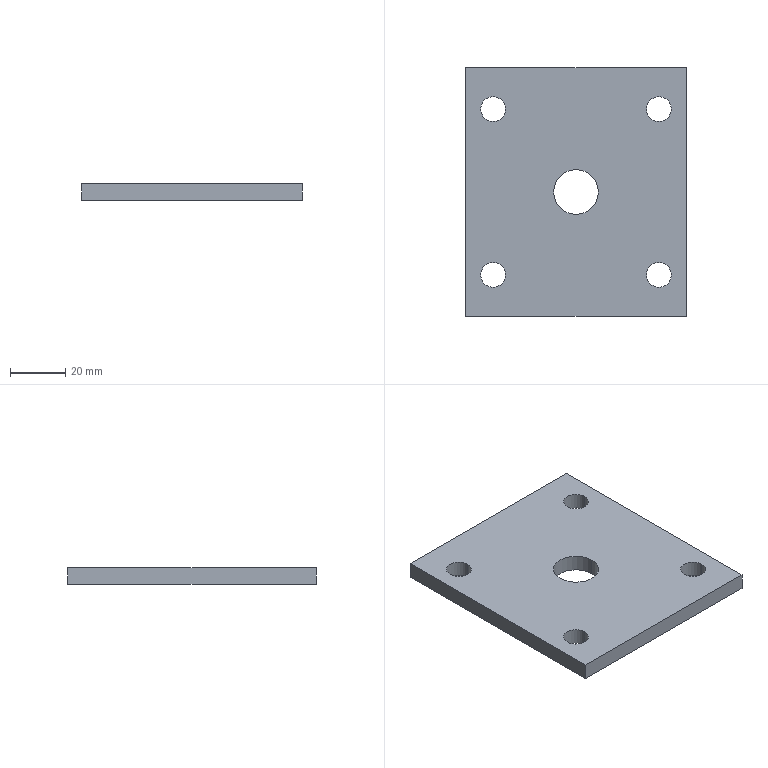Part | SolidWorks | features Extrusion 1, ICE 1 | 1 solid | 16 faces | box 80 x 90 x 6 mm | volume 40436 mm3 | cylinder 10 | plane 6 | commonest cylinder face diameters 9 x8 16.2 x2
STEP:
#1=CARTESIAN_POINT('',(-34.5,30.,-3.));
#2=VERTEX_POINT('',#1);
#3=CARTESIAN_POINT('',(-25.5,30.,-3.));
#4=VERTEX_POINT('',#3);
#5=CARTESIAN_POINT('',(-30.,30.,-3.));
#6=DIRECTION('',(0.,0.,1.));
#7=DIRECTION('',(1.,0.,0.));
#8=AXIS2_PLACEMENT_3D('',#5,#6,#7);
#9=CIRCLE('',#8,4.5);
#10=EDGE_CURVE('',#2,#4,#9,.T.);
#11=ORIENTED_EDGE('',*,*,#10,.F.);
#12=CARTESIAN_POINT('',(-34.5,30.,3.));
#13=VERTEX_POINT('',#12);
#14=CARTESIAN_POINT('',(-34.5,30.,-13.));
#15=DIRECTION('',(0.,0.,1.));
#16=VECTOR('',#15,1000.);
#17=LINE('',#14,#16);
#18=EDGE_CURVE('',#2,#13,#17,.T.);
#19=ORIENTED_EDGE('',*,*,#18,.T.);
#20=CARTESIAN_POINT('',(-25.5,30.,3.));
#21=VERTEX_POINT('',#20);
#22=CARTESIAN_POINT('',(-30.,30.,3.));
#23=DIRECTION('',(0.,0.,1.));
#24=DIRECTION('',(1.,0.,0.));
#25=AXIS2_PLACEMENT_3D('',#22,#23,#24);
#26=CIRCLE('',#25,4.5);
#27=EDGE_CURVE('',#13,#21,#26,.T.);
#28=ORIENTED_EDGE('',*,*,#27,.T.);
#29=CARTESIAN_POINT('',(-25.5,30.,-13.));
#30=DIRECTION('',(0.,0.,1.));
#31=VECTOR('',#30,1000.);
#32=LINE('',#29,#31);
#33=EDGE_CURVE('',#4,#21,#32,.T.);
#34=ORIENTED_EDGE('',*,*,#33,.F.);
#35=EDGE_LOOP('',(#11,#19,#28,#34));
#36=FACE_OUTER_BOUND('',#35,.T.);
#37=CARTESIAN_POINT('',(-30.,30.,-13.));
#38=DIRECTION('',(0.,0.,1.));
#39=DIRECTION('',(1.,0.,0.));
#40=AXIS2_PLACEMENT_3D('',#37,#38,#39);
#41=CYLINDRICAL_SURFACE('',#40,4.5);
#42=ADVANCED_FACE('',(#36),#41,.F.);
#43=CARTESIAN_POINT('',(25.5,-30.,-3.));
#44=VERTEX_POINT('',#43);
#45=CARTESIAN_POINT('',(34.5,-30.,-3.));
#46=VERTEX_POINT('',#45);
#47=CARTESIAN_POINT('',(30.,-30.,-3.));
#48=DIRECTION('',(0.,0.,1.));
#49=DIRECTION('',(1.,0.,0.));
#50=AXIS2_PLACEMENT_3D('',#47,#48,#49);
#51=CIRCLE('',#50,4.5);
#52=EDGE_CURVE('',#44,#46,#51,.T.);
#53=ORIENTED_EDGE('',*,*,#52,.F.);
#54=CARTESIAN_POINT('',(25.5,-30.,3.));
#55=VERTEX_POINT('',#54);
#56=CARTESIAN_POINT('',(25.5,-30.,-13.));
#57=DIRECTION('',(0.,0.,1.));
#58=VECTOR('',#57,1000.);
#59=LINE('',#56,#58);
#60=EDGE_CURVE('',#44,#55,#59,.T.);
#61=ORIENTED_EDGE('',*,*,#60,.T.);
#62=CARTESIAN_POINT('',(34.5,-30.,3.));
#63=VERTEX_POINT('',#62);
#64=CARTESIAN_POINT('',(30.,-30.,3.));
#65=DIRECTION('',(0.,0.,1.));
#66=DIRECTION('',(1.,0.,0.));
#67=AXIS2_PLACEMENT_3D('',#64,#65,#66);
#68=CIRCLE('',#67,4.5);
#69=EDGE_CURVE('',#55,#63,#68,.T.);
#70=ORIENTED_EDGE('',*,*,#69,.T.);
#71=CARTESIAN_POINT('',(34.5,-30.,-13.));
#72=DIRECTION('',(0.,0.,1.));
#73=VECTOR('',#72,1000.);
#74=LINE('',#71,#73);
#75=EDGE_CURVE('',#46,#63,#74,.T.);
#76=ORIENTED_EDGE('',*,*,#75,.F.);
#77=EDGE_LOOP('',(#53,#61,#70,#76));
#78=FACE_OUTER_BOUND('',#77,.T.);
#79=CARTESIAN_POINT('',(30.,-30.,-13.));
#80=DIRECTION('',(0.,0.,1.));
#81=DIRECTION('',(1.,0.,0.));
#82=AXIS2_PLACEMENT_3D('',#79,#80,#81);
#83=CYLINDRICAL_SURFACE('',#82,4.5);
#84=ADVANCED_FACE('',(#78),#83,.F.);
#85=CARTESIAN_POINT('',(25.5,30.,-3.));
#86=VERTEX_POINT('',#85);
#87=CARTESIAN_POINT('',(34.5,30.,-3.));
#88=VERTEX_POINT('',#87);
#89=CARTESIAN_POINT('',(30.,30.,-3.));
#90=DIRECTION('',(0.,0.,1.));
#91=DIRECTION('',(1.,0.,0.));
#92=AXIS2_PLACEMENT_3D('',#89,#90,#91);
#93=CIRCLE('',#92,4.5);
#94=EDGE_CURVE('',#86,#88,#93,.T.);
#95=ORIENTED_EDGE('',*,*,#94,.F.);
#96=CARTESIAN_POINT('',(25.5,30.,3.));
#97=VERTEX_POINT('',#96);
#98=CARTESIAN_POINT('',(25.5,30.,-13.));
#99=DIRECTION('',(0.,0.,1.));
#100=VECTOR('',#99,1000.);
#101=LINE('',#98,#100);
#102=EDGE_CURVE('',#86,#97,#101,.T.);
#103=ORIENTED_EDGE('',*,*,#102,.T.);
#104=CARTESIAN_POINT('',(34.5,30.,3.));
#105=VERTEX_POINT('',#104);
#106=CARTESIAN_POINT('',(30.,30.,3.));
#107=DIRECTION('',(0.,0.,1.));
#108=DIRECTION('',(1.,0.,0.));
#109=AXIS2_PLACEMENT_3D('',#106,#107,#108);
#110=CIRCLE('',#109,4.5);
#111=EDGE_CURVE('',#97,#105,#110,.T.);
#112=ORIENTED_EDGE('',*,*,#111,.T.);
#113=CARTESIAN_POINT('',(34.5,30.,-13.));
#114=DIRECTION('',(0.,0.,1.));
#115=VECTOR('',#114,1000.);
#116=LINE('',#113,#115);
#117=EDGE_CURVE('',#88,#105,#116,.T.);
#118=ORIENTED_EDGE('',*,*,#117,.F.);
#119=EDGE_LOOP('',(#95,#103,#112,#118));
#120=FACE_OUTER_BOUND('',#119,.T.);
#121=CARTESIAN_POINT('',(30.,30.,-13.));
#122=DIRECTION('',(0.,0.,1.));
#123=DIRECTION('',(1.,0.,0.));
#124=AXIS2_PLACEMENT_3D('',#121,#122,#123);
#125=CYLINDRICAL_SURFACE('',#124,4.5);
#126=ADVANCED_FACE('',(#120),#125,.F.);
#127=CARTESIAN_POINT('',(-8.1,0.,-3.));
#128=VERTEX_POINT('',#127);
#129=CARTESIAN_POINT('',(8.1,0.,-3.));
#130=VERTEX_POINT('',#129);
#131=CARTESIAN_POINT('',(0.,0.,-3.));
#132=DIRECTION('',(0.,0.,1.));
#133=DIRECTION('',(1.,0.,0.));
#134=AXIS2_PLACEMENT_3D('',#131,#132,#133);
#135=CIRCLE('',#134,8.1);
#136=EDGE_CURVE('',#128,#130,#135,.T.);
#137=ORIENTED_EDGE('',*,*,#136,.F.);
#138=CARTESIAN_POINT('',(-8.1,0.,3.));
#139=VERTEX_POINT('',#138);
#140=CARTESIAN_POINT('',(-8.1,0.,-13.));
#141=DIRECTION('',(0.,0.,1.));
#142=VECTOR('',#141,1000.);
#143=LINE('',#140,#142);
#144=EDGE_CURVE('',#128,#139,#143,.T.);
#145=ORIENTED_EDGE('',*,*,#144,.T.);
#146=CARTESIAN_POINT('',(8.1,0.,3.));
#147=VERTEX_POINT('',#146);
#148=CARTESIAN_POINT('',(0.,0.,3.));
#149=DIRECTION('',(0.,0.,1.));
#150=DIRECTION('',(1.,0.,0.));
#151=AXIS2_PLACEMENT_3D('',#148,#149,#150);
#152=CIRCLE('',#151,8.1);
#153=EDGE_CURVE('',#139,#147,#152,.T.);
#154=ORIENTED_EDGE('',*,*,#153,.T.);
#155=CARTESIAN_POINT('',(8.1,0.,-13.));
#156=DIRECTION('',(0.,0.,1.));
#157=VECTOR('',#156,1000.);
#158=LINE('',#155,#157);
#159=EDGE_CURVE('',#130,#147,#158,.T.);
#160=ORIENTED_EDGE('',*,*,#159,.F.);
#161=EDGE_LOOP('',(#137,#145,#154,#160));
#162=FACE_OUTER_BOUND('',#161,.T.);
#163=CARTESIAN_POINT('',(0.,0.,-13.));
#164=DIRECTION('',(0.,0.,1.));
#165=DIRECTION('',(1.,0.,0.));
#166=AXIS2_PLACEMENT_3D('',#163,#164,#165);
#167=CYLINDRICAL_SURFACE('',#166,8.1);
#168=ADVANCED_FACE('',(#162),#167,.F.);
#169=CARTESIAN_POINT('',(-34.5,-30.,-3.));
#170=VERTEX_POINT('',#169);
#171=CARTESIAN_POINT('',(-25.5,-30.,-3.));
#172=VERTEX_POINT('',#171);
#173=CARTESIAN_POINT('',(-30.,-30.,-3.));
#174=DIRECTION('',(0.,0.,1.));
#175=DIRECTION('',(1.,0.,0.));
#176=AXIS2_PLACEMENT_3D('',#173,#174,#175);
#177=CIRCLE('',#176,4.5);
#178=EDGE_CURVE('',#170,#172,#177,.T.);
#179=ORIENTED_EDGE('',*,*,#178,.F.);
#180=CARTESIAN_POINT('',(-34.5,-30.,3.));
#181=VERTEX_POINT('',#180);
#182=CARTESIAN_POINT('',(-34.5,-30.,-13.));
#183=DIRECTION('',(0.,0.,1.));
#184=VECTOR('',#183,1000.);
#185=LINE('',#182,#184);
#186=EDGE_CURVE('',#170,#181,#185,.T.);
#187=ORIENTED_EDGE('',*,*,#186,.T.);
#188=CARTESIAN_POINT('',(-25.5,-30.,3.));
#189=VERTEX_POINT('',#188);
#190=CARTESIAN_POINT('',(-30.,-30.,3.));
#191=DIRECTION('',(0.,0.,1.));
#192=DIRECTION('',(1.,0.,0.));
#193=AXIS2_PLACEMENT_3D('',#190,#191,#192);
#194=CIRCLE('',#193,4.5);
#195=EDGE_CURVE('',#181,#189,#194,.T.);
#196=ORIENTED_EDGE('',*,*,#195,.T.);
#197=CARTESIAN_POINT('',(-25.5,-30.,-13.));
#198=DIRECTION('',(0.,0.,1.));
#199=VECTOR('',#198,1000.);
#200=LINE('',#197,#199);
#201=EDGE_CURVE('',#172,#189,#200,.T.);
#202=ORIENTED_EDGE('',*,*,#201,.F.);
#203=EDGE_LOOP('',(#179,#187,#196,#202));
#204=FACE_OUTER_BOUND('',#203,.T.);
#205=CARTESIAN_POINT('',(-30.,-30.,-13.));
#206=DIRECTION('',(0.,0.,1.));
#207=DIRECTION('',(1.,0.,0.));
#208=AXIS2_PLACEMENT_3D('',#205,#206,#207);
#209=CYLINDRICAL_SURFACE('',#208,4.5);
#210=ADVANCED_FACE('',(#204),#209,.F.);
#211=CARTESIAN_POINT('',(-40.,45.,3.));
#212=VERTEX_POINT('',#211);
#213=CARTESIAN_POINT('',(-40.,-45.,3.));
#214=VERTEX_POINT('',#213);
#215=CARTESIAN_POINT('',(-40.,45.,3.));
#216=DIRECTION('',(0.,-1.,0.));
#217=VECTOR('',#216,1000.);
#218=LINE('',#215,#217);
#219=EDGE_CURVE('',#212,#214,#218,.T.);
#220=ORIENTED_EDGE('',*,*,#219,.F.);
#221=CARTESIAN_POINT('',(-40.,45.,-3.));
#222=VERTEX_POINT('',#221);
#223=CARTESIAN_POINT('',(-40.,45.,-3.));
#224=DIRECTION('',(0.,0.,1.));
#225=VECTOR('',#224,1000.);
#226=LINE('',#223,#225);
#227=EDGE_CURVE('',#222,#212,#226,.T.);
#228=ORIENTED_EDGE('',*,*,#227,.F.);
#229=CARTESIAN_POINT('',(-40.,-45.,-3.));
#230=VERTEX_POINT('',#229);
#231=CARTESIAN_POINT('',(-40.,45.,-3.));
#232=DIRECTION('',(0.,-1.,0.));
#233=VECTOR('',#232,1000.);
#234=LINE('',#231,#233);
#235=EDGE_CURVE('',#222,#230,#234,.T.);
#236=ORIENTED_EDGE('',*,*,#235,.T.);
#237=CARTESIAN_POINT('',(-40.,-45.,-3.));
#238=DIRECTION('',(0.,0.,1.));
#239=VECTOR('',#238,1000.);
#240=LINE('',#237,#239);
#241=EDGE_CURVE('',#230,#214,#240,.T.);
#242=ORIENTED_EDGE('',*,*,#241,.T.);
#243=EDGE_LOOP('',(#220,#228,#236,#242));
#244=FACE_OUTER_BOUND('',#243,.T.);
#245=CARTESIAN_POINT('',(-40.,45.,-3.));
#246=DIRECTION('',(-1.,0.,0.));
#247=DIRECTION('',(0.,0.,1.));
#248=AXIS2_PLACEMENT_3D('',#245,#246,#247);
#249=PLANE('',#248);
#250=ADVANCED_FACE('',(#244),#249,.T.);
#251=CARTESIAN_POINT('',(40.,45.,3.));
#252=VERTEX_POINT('',#251);
#253=CARTESIAN_POINT('',(40.,45.,3.));
#254=DIRECTION('',(-1.,0.,0.));
#255=VECTOR('',#254,1000.);
#256=LINE('',#253,#255);
#257=EDGE_CURVE('',#252,#212,#256,.T.);
#258=ORIENTED_EDGE('',*,*,#257,.F.);
#259=CARTESIAN_POINT('',(40.,45.,-3.));
#260=VERTEX_POINT('',#259);
#261=CARTESIAN_POINT('',(40.,45.,-3.));
#262=DIRECTION('',(0.,0.,1.));
#263=VECTOR('',#262,1000.);
#264=LINE('',#261,#263);
#265=EDGE_CURVE('',#260,#252,#264,.T.);
#266=ORIENTED_EDGE('',*,*,#265,.F.);
#267=CARTESIAN_POINT('',(40.,45.,-3.));
#268=DIRECTION('',(-1.,0.,0.));
#269=VECTOR('',#268,1000.);
#270=LINE('',#267,#269);
#271=EDGE_CURVE('',#260,#222,#270,.T.);
#272=ORIENTED_EDGE('',*,*,#271,.T.);
#273=ORIENTED_EDGE('',*,*,#227,.T.);
#274=EDGE_LOOP('',(#258,#266,#272,#273));
#275=FACE_OUTER_BOUND('',#274,.T.);
#276=CARTESIAN_POINT('',(40.,45.,-3.));
#277=DIRECTION('',(0.,1.,0.));
#278=DIRECTION('',(0.,0.,1.));
#279=AXIS2_PLACEMENT_3D('',#276,#277,#278);
#280=PLANE('',#279);
#281=ADVANCED_FACE('',(#275),#280,.T.);
#282=CARTESIAN_POINT('',(40.,-45.,3.));
#283=VERTEX_POINT('',#282);
#284=CARTESIAN_POINT('',(40.,-45.,3.));
#285=DIRECTION('',(0.,1.,0.));
#286=VECTOR('',#285,1000.);
#287=LINE('',#284,#286);
#288=EDGE_CURVE('',#283,#252,#287,.T.);
#289=ORIENTED_EDGE('',*,*,#288,.F.);
#290=CARTESIAN_POINT('',(40.,-45.,-3.));
#291=VERTEX_POINT('',#290);
#292=CARTESIAN_POINT('',(40.,-45.,-3.));
#293=DIRECTION('',(0.,0.,1.));
#294=VECTOR('',#293,1000.);
#295=LINE('',#292,#294);
#296=EDGE_CURVE('',#291,#283,#295,.T.);
#297=ORIENTED_EDGE('',*,*,#296,.F.);
#298=CARTESIAN_POINT('',(40.,-45.,-3.));
#299=DIRECTION('',(0.,1.,0.));
#300=VECTOR('',#299,1000.);
#301=LINE('',#298,#300);
#302=EDGE_CURVE('',#291,#260,#301,.T.);
#303=ORIENTED_EDGE('',*,*,#302,.T.);
#304=ORIENTED_EDGE('',*,*,#265,.T.);
#305=EDGE_LOOP('',(#289,#297,#303,#304));
#306=FACE_OUTER_BOUND('',#305,.T.);
#307=CARTESIAN_POINT('',(40.,-45.,-3.));
#308=DIRECTION('',(1.,0.,0.));
#309=DIRECTION('',(0.,0.,-1.));
#310=AXIS2_PLACEMENT_3D('',#307,#308,#309);
#311=PLANE('',#310);
#312=ADVANCED_FACE('',(#306),#311,.T.);
#313=CARTESIAN_POINT('',(-40.,-45.,3.));
#314=DIRECTION('',(1.,0.,0.));
#315=VECTOR('',#314,1000.);
#316=LINE('',#313,#315);
#317=EDGE_CURVE('',#214,#283,#316,.T.);
#318=ORIENTED_EDGE('',*,*,#317,.F.);
#319=ORIENTED_EDGE('',*,*,#241,.F.);
#320=CARTESIAN_POINT('',(-40.,-45.,-3.));
#321=DIRECTION('',(1.,0.,0.));
#322=VECTOR('',#321,1000.);
#323=LINE('',#320,#322);
#324=EDGE_CURVE('',#230,#291,#323,.T.);
#325=ORIENTED_EDGE('',*,*,#324,.T.);
#326=ORIENTED_EDGE('',*,*,#296,.T.);
#327=EDGE_LOOP('',(#318,#319,#325,#326));
#328=FACE_OUTER_BOUND('',#327,.T.);
#329=CARTESIAN_POINT('',(-40.,-45.,-3.));
#330=DIRECTION('',(0.,-1.,0.));
#331=DIRECTION('',(0.,0.,-1.));
#332=AXIS2_PLACEMENT_3D('',#329,#330,#331);
#333=PLANE('',#332);
#334=ADVANCED_FACE('',(#328),#333,.T.);
#335=CARTESIAN_POINT('',(-30.,30.,-3.));
#336=DIRECTION('',(0.,0.,1.));
#337=DIRECTION('',(1.,0.,0.));
#338=AXIS2_PLACEMENT_3D('',#335,#336,#337);
#339=CIRCLE('',#338,4.5);
#340=EDGE_CURVE('',#4,#2,#339,.T.);
#341=ORIENTED_EDGE('',*,*,#340,.T.);
#342=ORIENTED_EDGE('',*,*,#10,.T.);
#343=EDGE_LOOP('',(#341,#342));
#344=FACE_BOUND('',#343,.T.);
#345=CARTESIAN_POINT('',(30.,-30.,-3.));
#346=DIRECTION('',(0.,0.,1.));
#347=DIRECTION('',(1.,0.,0.));
#348=AXIS2_PLACEMENT_3D('',#345,#346,#347);
#349=CIRCLE('',#348,4.5);
#350=EDGE_CURVE('',#46,#44,#349,.T.);
#351=ORIENTED_EDGE('',*,*,#350,.T.);
#352=ORIENTED_EDGE('',*,*,#52,.T.);
#353=EDGE_LOOP('',(#351,#352));
#354=FACE_BOUND('',#353,.T.);
#355=CARTESIAN_POINT('',(30.,30.,-3.));
#356=DIRECTION('',(0.,0.,1.));
#357=DIRECTION('',(1.,0.,0.));
#358=AXIS2_PLACEMENT_3D('',#355,#356,#357);
#359=CIRCLE('',#358,4.5);
#360=EDGE_CURVE('',#88,#86,#359,.T.);
#361=ORIENTED_EDGE('',*,*,#360,.T.);
#362=ORIENTED_EDGE('',*,*,#94,.T.);
#363=EDGE_LOOP('',(#361,#362));
#364=FACE_BOUND('',#363,.T.);
#365=CARTESIAN_POINT('',(0.,0.,-3.));
#366=DIRECTION('',(0.,0.,1.));
#367=DIRECTION('',(1.,0.,0.));
#368=AXIS2_PLACEMENT_3D('',#365,#366,#367);
#369=CIRCLE('',#368,8.1);
#370=EDGE_CURVE('',#130,#128,#369,.T.);
#371=ORIENTED_EDGE('',*,*,#370,.T.);
#372=ORIENTED_EDGE('',*,*,#136,.T.);
#373=EDGE_LOOP('',(#371,#372));
#374=FACE_BOUND('',#373,.T.);
#375=CARTESIAN_POINT('',(-30.,-30.,-3.));
#376=DIRECTION('',(0.,0.,1.));
#377=DIRECTION('',(1.,0.,0.));
#378=AXIS2_PLACEMENT_3D('',#375,#376,#377);
#379=CIRCLE('',#378,4.5);
#380=EDGE_CURVE('',#172,#170,#379,.T.);
#381=ORIENTED_EDGE('',*,*,#380,.T.);
#382=ORIENTED_EDGE('',*,*,#178,.T.);
#383=EDGE_LOOP('',(#381,#382));
#384=FACE_BOUND('',#383,.T.);
#385=ORIENTED_EDGE('',*,*,#235,.F.);
#386=ORIENTED_EDGE('',*,*,#271,.F.);
#387=ORIENTED_EDGE('',*,*,#302,.F.);
#388=ORIENTED_EDGE('',*,*,#324,.F.);
#389=EDGE_LOOP('',(#385,#386,#387,#388));
#390=FACE_OUTER_BOUND('',#389,.T.);
#391=CARTESIAN_POINT('',(0.,0.,-3.));
#392=DIRECTION('',(0.,0.,1.));
#393=DIRECTION('',(1.,0.,0.));
#394=AXIS2_PLACEMENT_3D('',#391,#392,#393);
#395=PLANE('',#394);
#396=ADVANCED_FACE('',(#344,#354,#364,#374,#384,#390),#395,.F.);
#397=CARTESIAN_POINT('',(-30.,30.,3.));
#398=DIRECTION('',(0.,0.,1.));
#399=DIRECTION('',(1.,0.,0.));
#400=AXIS2_PLACEMENT_3D('',#397,#398,#399);
#401=CIRCLE('',#400,4.5);
#402=EDGE_CURVE('',#21,#13,#401,.T.);
#403=ORIENTED_EDGE('',*,*,#402,.F.);
#404=ORIENTED_EDGE('',*,*,#27,.F.);
#405=EDGE_LOOP('',(#403,#404));
#406=FACE_BOUND('',#405,.T.);
#407=CARTESIAN_POINT('',(30.,-30.,3.));
#408=DIRECTION('',(0.,0.,1.));
#409=DIRECTION('',(1.,0.,0.));
#410=AXIS2_PLACEMENT_3D('',#407,#408,#409);
#411=CIRCLE('',#410,4.5);
#412=EDGE_CURVE('',#63,#55,#411,.T.);
#413=ORIENTED_EDGE('',*,*,#412,.F.);
#414=ORIENTED_EDGE('',*,*,#69,.F.);
#415=EDGE_LOOP('',(#413,#414));
#416=FACE_BOUND('',#415,.T.);
#417=CARTESIAN_POINT('',(30.,30.,3.));
#418=DIRECTION('',(0.,0.,1.));
#419=DIRECTION('',(1.,0.,0.));
#420=AXIS2_PLACEMENT_3D('',#417,#418,#419);
#421=CIRCLE('',#420,4.5);
#422=EDGE_CURVE('',#105,#97,#421,.T.);
#423=ORIENTED_EDGE('',*,*,#422,.F.);
#424=ORIENTED_EDGE('',*,*,#111,.F.);
#425=EDGE_LOOP('',(#423,#424));
#426=FACE_BOUND('',#425,.T.);
#427=CARTESIAN_POINT('',(0.,0.,3.));
#428=DIRECTION('',(0.,0.,1.));
#429=DIRECTION('',(1.,0.,0.));
#430=AXIS2_PLACEMENT_3D('',#427,#428,#429);
#431=CIRCLE('',#430,8.1);
#432=EDGE_CURVE('',#147,#139,#431,.T.);
#433=ORIENTED_EDGE('',*,*,#432,.F.);
#434=ORIENTED_EDGE('',*,*,#153,.F.);
#435=EDGE_LOOP('',(#433,#434));
#436=FACE_BOUND('',#435,.T.);
#437=CARTESIAN_POINT('',(-30.,-30.,3.));
#438=DIRECTION('',(0.,0.,1.));
#439=DIRECTION('',(1.,0.,0.));
#440=AXIS2_PLACEMENT_3D('',#437,#438,#439);
#441=CIRCLE('',#440,4.5);
#442=EDGE_CURVE('',#189,#181,#441,.T.);
#443=ORIENTED_EDGE('',*,*,#442,.F.);
#444=ORIENTED_EDGE('',*,*,#195,.F.);
#445=EDGE_LOOP('',(#443,#444));
#446=FACE_BOUND('',#445,.T.);
#447=ORIENTED_EDGE('',*,*,#219,.T.);
#448=ORIENTED_EDGE('',*,*,#317,.T.);
#449=ORIENTED_EDGE('',*,*,#288,.T.);
#450=ORIENTED_EDGE('',*,*,#257,.T.);
#451=EDGE_LOOP('',(#447,#448,#449,#450));
#452=FACE_OUTER_BOUND('',#451,.T.);
#453=CARTESIAN_POINT('',(0.,0.,3.));
#454=DIRECTION('',(0.,0.,1.));
#455=DIRECTION('',(1.,0.,0.));
#456=AXIS2_PLACEMENT_3D('',#453,#454,#455);
#457=PLANE('',#456);
#458=ADVANCED_FACE('',(#406,#416,#426,#436,#446,#452),#457,.T.);
#459=ORIENTED_EDGE('',*,*,#186,.F.);
#460=ORIENTED_EDGE('',*,*,#380,.F.);
#461=ORIENTED_EDGE('',*,*,#201,.T.);
#462=ORIENTED_EDGE('',*,*,#442,.T.);
#463=EDGE_LOOP('',(#459,#460,#461,#462));
#464=FACE_OUTER_BOUND('',#463,.T.);
#465=CARTESIAN_POINT('',(-30.,-30.,-13.));
#466=DIRECTION('',(0.,0.,1.));
#467=DIRECTION('',(1.,0.,0.));
#468=AXIS2_PLACEMENT_3D('',#465,#466,#467);
#469=CYLINDRICAL_SURFACE('',#468,4.5);
#470=ADVANCED_FACE('',(#464),#469,.F.);
#471=ORIENTED_EDGE('',*,*,#144,.F.);
#472=ORIENTED_EDGE('',*,*,#370,.F.);
#473=ORIENTED_EDGE('',*,*,#159,.T.);
#474=ORIENTED_EDGE('',*,*,#432,.T.);
#475=EDGE_LOOP('',(#471,#472,#473,#474));
#476=FACE_OUTER_BOUND('',#475,.T.);
#477=CARTESIAN_POINT('',(0.,0.,-13.));
#478=DIRECTION('',(0.,0.,1.));
#479=DIRECTION('',(1.,0.,0.));
#480=AXIS2_PLACEMENT_3D('',#477,#478,#479);
#481=CYLINDRICAL_SURFACE('',#480,8.1);
#482=ADVANCED_FACE('',(#476),#481,.F.);
#483=ORIENTED_EDGE('',*,*,#102,.F.);
#484=ORIENTED_EDGE('',*,*,#360,.F.);
#485=ORIENTED_EDGE('',*,*,#117,.T.);
#486=ORIENTED_EDGE('',*,*,#422,.T.);
#487=EDGE_LOOP('',(#483,#484,#485,#486));
#488=FACE_OUTER_BOUND('',#487,.T.);
#489=CARTESIAN_POINT('',(30.,30.,-13.));
#490=DIRECTION('',(0.,0.,1.));
#491=DIRECTION('',(1.,0.,0.));
#492=AXIS2_PLACEMENT_3D('',#489,#490,#491);
#493=CYLINDRICAL_SURFACE('',#492,4.5);
#494=ADVANCED_FACE('',(#488),#493,.F.);
#495=ORIENTED_EDGE('',*,*,#60,.F.);
#496=ORIENTED_EDGE('',*,*,#350,.F.);
#497=ORIENTED_EDGE('',*,*,#75,.T.);
#498=ORIENTED_EDGE('',*,*,#412,.T.);
#499=EDGE_LOOP('',(#495,#496,#497,#498));
#500=FACE_OUTER_BOUND('',#499,.T.);
#501=CARTESIAN_POINT('',(30.,-30.,-13.));
#502=DIRECTION('',(0.,0.,1.));
#503=DIRECTION('',(1.,0.,0.));
#504=AXIS2_PLACEMENT_3D('',#501,#502,#503);
#505=CYLINDRICAL_SURFACE('',#504,4.5);
#506=ADVANCED_FACE('',(#500),#505,.F.);
#507=ORIENTED_EDGE('',*,*,#18,.F.);
#508=ORIENTED_EDGE('',*,*,#340,.F.);
#509=ORIENTED_EDGE('',*,*,#33,.T.);
#510=ORIENTED_EDGE('',*,*,#402,.T.);
#511=EDGE_LOOP('',(#507,#508,#509,#510));
#512=FACE_OUTER_BOUND('',#511,.T.);
#513=CARTESIAN_POINT('',(-30.,30.,-13.));
#514=DIRECTION('',(0.,0.,1.));
#515=DIRECTION('',(1.,0.,0.));
#516=AXIS2_PLACEMENT_3D('',#513,#514,#515);
#517=CYLINDRICAL_SURFACE('',#516,4.5);
#518=ADVANCED_FACE('',(#512),#517,.F.);
#519=CLOSED_SHELL('',(#42,#84,#126,#168,#210,#250,#281,#312,#334,#396,#458,#470,#482,#494,#506,#518));
#520=MANIFOLD_SOLID_BREP('',#519);
#521=CARTESIAN_POINT('',(0.,0.,0.));
#522=DIRECTION('',(0.,0.,1.));
#523=DIRECTION('',(1.,0.,0.));
#524=AXIS2_PLACEMENT_3D('',#521,#522,#523);
#525=(LENGTH_UNIT()NAMED_UNIT(*)SI_UNIT(.MILLI.,.METRE.));
#526=UNCERTAINTY_MEASURE_WITH_UNIT(LENGTH_MEASURE(0.00001),#525,'','');
#527=(NAMED_UNIT(*)PLANE_ANGLE_UNIT()SI_UNIT($,.RADIAN.));
#528=(NAMED_UNIT(*)SI_UNIT($,.STERADIAN.)SOLID_ANGLE_UNIT());
#529=(GEOMETRIC_REPRESENTATION_CONTEXT(3)GLOBAL_UNCERTAINTY_ASSIGNED_CONTEXT((#526))GLOBAL_UNIT_ASSIGNED_CONTEXT((#525,#527,#528))REPRESENTATION_CONTEXT('',''));
#530=ADVANCED_BREP_SHAPE_REPRESENTATION('',(#520,#524),#529);